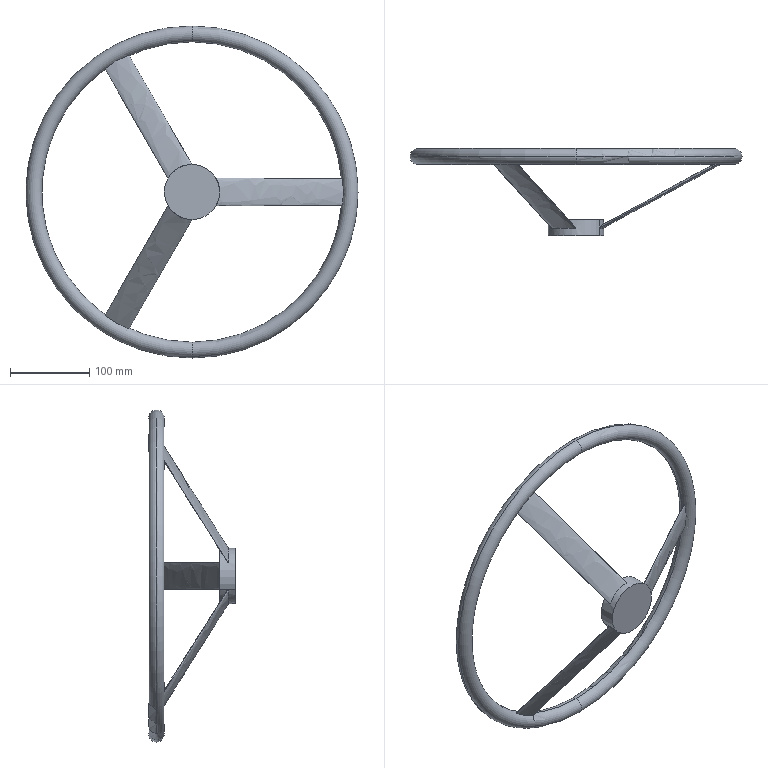Part | SolidWorks | 1 solid | 17 faces | box 420 x 110 x 420 mm | volume 545281 mm3 | spline 6 | plane 5 | torus 4 | cylinder 2 | commonest cylinder face diameters 70 x2
STEP:
#1=CARTESIAN_POINT('',(-101.45,99.061,160.701));
#2=VERTEX_POINT('',#1);
#3=CARTESIAN_POINT('',(-88.446,99.061,168.208));
#4=VERTEX_POINT('',#3);
#5=CARTESIAN_POINT('',(-101.45,99.061,160.701));
#6=CARTESIAN_POINT('',(-100.399,98.952,161.376));
#7=CARTESIAN_POINT('',(-99.34,98.865,162.042));
#8=CARTESIAN_POINT('',(-97.203,98.749,163.349));
#9=CARTESIAN_POINT('',(-96.124,98.719,163.991));
#10=CARTESIAN_POINT('',(-92.865,98.719,165.873));
#11=CARTESIAN_POINT('',(-90.666,98.842,167.065));
#12=CARTESIAN_POINT('',(-88.446,99.061,168.208));
#13=B_SPLINE_CURVE_WITH_KNOTS('',3,(#5,#6,#7,#8,#9,#10,#11,#12),.UNSPECIFIED.,.F.,.F.,(4,2,2,4),(0.002179,0.00594,0.009701,0.01722),.UNSPECIFIED.);
#14=EDGE_CURVE('',#2,#4,#13,.T.);
#15=ORIENTED_EDGE('',*,*,#14,.F.);
#16=CARTESIAN_POINT('',(-110.077,96.46,155.659));
#17=VERTEX_POINT('',#16);
#18=CARTESIAN_POINT('',(-110.077,96.46,155.659));
#19=CARTESIAN_POINT('',(-110.067,96.511,155.642));
#20=CARTESIAN_POINT('',(-110.046,96.564,155.633));
#21=CARTESIAN_POINT('',(-109.992,96.661,155.628));
#22=CARTESIAN_POINT('',(-109.959,96.706,155.632));
#23=CARTESIAN_POINT('',(-109.851,96.831,155.656));
#24=CARTESIAN_POINT('',(-109.769,96.901,155.686));
#25=CARTESIAN_POINT('',(-109.519,97.09,155.788));
#26=CARTESIAN_POINT('',(-109.341,97.191,155.877));
#27=CARTESIAN_POINT('',(-108.808,97.463,156.156));
#28=CARTESIAN_POINT('',(-108.445,97.604,156.366));
#29=CARTESIAN_POINT('',(-107.718,97.857,156.796));
#30=CARTESIAN_POINT('',(-107.354,97.967,157.018));
#31=CARTESIAN_POINT('',(-106.623,98.167,157.467));
#32=CARTESIAN_POINT('',(-106.256,98.257,157.695));
#33=CARTESIAN_POINT('',(-105.155,98.506,158.383));
#34=CARTESIAN_POINT('',(-104.418,98.644,158.847));
#35=CARTESIAN_POINT('',(-102.939,98.88,159.775));
#36=CARTESIAN_POINT('',(-102.196,98.979,160.239));
#37=CARTESIAN_POINT('',(-101.45,99.061,160.701));
#38=B_SPLINE_CURVE_WITH_KNOTS('',3,(#18,#19,#20,#21,#22,#23,#24,#25,#26,#27,#28,#29,#30,#31,#32,#33,#34,#35,#36,#37),.UNSPECIFIED.,.F.,.F.,(4,2,2,2,2,2,2,2,2,4),(0.04636,0.04653,0.04669,0.04702,0.04768,0.049,0.05032,0.05164,0.05428,0.05692),.UNSPECIFIED.);
#39=EDGE_CURVE('',#17,#2,#38,.T.);
#40=ORIENTED_EDGE('',*,*,#39,.F.);
#41=CARTESIAN_POINT('',(-79.766,96.46,173.159));
#42=VERTEX_POINT('',#41);
#43=CARTESIAN_POINT('',(-79.766,96.46,173.159));
#44=CARTESIAN_POINT('',(-79.783,96.371,173.188));
#45=CARTESIAN_POINT('',(-79.837,96.286,173.2));
#46=CARTESIAN_POINT('',(-79.968,96.149,173.201));
#47=CARTESIAN_POINT('',(-80.045,96.092,173.192));
#48=CARTESIAN_POINT('',(-80.282,95.943,173.153));
#49=CARTESIAN_POINT('',(-80.453,95.869,173.111));
#50=CARTESIAN_POINT('',(-80.963,95.674,172.973));
#51=CARTESIAN_POINT('',(-81.309,95.584,172.86));
#52=CARTESIAN_POINT('',(-82.001,95.425,172.621));
#53=CARTESIAN_POINT('',(-82.349,95.36,172.493));
#54=CARTESIAN_POINT('',(-83.042,95.245,172.228));
#55=CARTESIAN_POINT('',(-83.388,95.196,172.091));
#56=CARTESIAN_POINT('',(-84.424,95.062,171.669));
#57=CARTESIAN_POINT('',(-85.111,94.992,171.374));
#58=CARTESIAN_POINT('',(-86.479,94.875,170.765));
#59=CARTESIAN_POINT('',(-87.159,94.827,170.451));
#60=CARTESIAN_POINT('',(-89.191,94.707,169.486));
#61=CARTESIAN_POINT('',(-90.532,94.655,168.81));
#62=CARTESIAN_POINT('',(-93.188,94.587,167.409));
#63=CARTESIAN_POINT('',(-94.502,94.571,166.682));
#64=CARTESIAN_POINT('',(-97.103,94.571,165.18));
#65=CARTESIAN_POINT('',(-98.39,94.587,164.405));
#66=CARTESIAN_POINT('',(-100.931,94.655,162.806));
#67=CARTESIAN_POINT('',(-102.187,94.707,161.982));
#68=CARTESIAN_POINT('',(-104.039,94.828,160.706));
#69=CARTESIAN_POINT('',(-104.651,94.875,160.273));
#70=CARTESIAN_POINT('',(-105.862,94.993,159.393));
#71=CARTESIAN_POINT('',(-106.46,95.062,158.946));
#72=CARTESIAN_POINT('',(-107.344,95.196,158.26));
#73=CARTESIAN_POINT('',(-107.636,95.246,158.028));
#74=CARTESIAN_POINT('',(-108.212,95.361,157.56));
#75=CARTESIAN_POINT('',(-108.496,95.426,157.323));
#76=CARTESIAN_POINT('',(-108.912,95.545,156.962));
#77=CARTESIAN_POINT('',(-109.048,95.588,156.841));
#78=CARTESIAN_POINT('',(-109.316,95.687,156.597));
#79=CARTESIAN_POINT('',(-109.447,95.741,156.474));
#80=CARTESIAN_POINT('',(-109.697,95.871,156.225));
#81=CARTESIAN_POINT('',(-109.817,95.945,156.099));
#82=CARTESIAN_POINT('',(-109.969,96.095,155.914));
#83=CARTESIAN_POINT('',(-110.015,96.152,155.852));
#84=CARTESIAN_POINT('',(-110.078,96.288,155.74));
#85=CARTESIAN_POINT('',(-110.094,96.372,155.688));
#86=CARTESIAN_POINT('',(-110.077,96.46,155.659));
#87=B_SPLINE_CURVE_WITH_KNOTS('',3,(#43,#44,#45,#46,#47,#48,#49,#50,#51,#52,#53,#54,#55,#56,#57,#58,#59,#60,#61,#62,#63,#64,#65,#66,#67,#68,#69,#70,#71,#72,#73,#74,#75,#76,#77,#78,#79,#80,#81,#82,#83,#84,#85,#86),.UNSPECIFIED.,.F.,.F.,(4,2,2,2,2,2,2,2,2,2,2,2,2,2,2,2,2,2,2,2,2,4),(0.01057,0.01085,0.01113,0.01169,0.01281,0.01393,0.01505,0.01728,0.01952,0.02399,0.02847,0.03294,0.03742,0.03965,0.04189,0.04301,0.04413,0.04469,0.04525,0.04581,0.04609,0.04636),.UNSPECIFIED.);
#88=EDGE_CURVE('',#42,#17,#87,.T.);
#89=ORIENTED_EDGE('',*,*,#88,.F.);
#90=CARTESIAN_POINT('',(-88.446,99.061,168.208));
#91=CARTESIAN_POINT('',(-87.673,98.979,168.624));
#92=CARTESIAN_POINT('',(-86.9,98.88,169.035));
#93=CARTESIAN_POINT('',(-85.357,98.644,169.852));
#94=CARTESIAN_POINT('',(-84.587,98.506,170.258));
#95=CARTESIAN_POINT('',(-83.441,98.258,170.868));
#96=CARTESIAN_POINT('',(-83.061,98.167,171.071));
#97=CARTESIAN_POINT('',(-82.306,97.967,171.479));
#98=CARTESIAN_POINT('',(-81.931,97.857,171.684));
#99=CARTESIAN_POINT('',(-81.381,97.668,171.994));
#100=CARTESIAN_POINT('',(-81.199,97.601,172.098));
#101=CARTESIAN_POINT('',(-80.841,97.453,172.308));
#102=CARTESIAN_POINT('',(-80.664,97.373,172.415));
#103=CARTESIAN_POINT('',(-80.325,97.192,172.629));
#104=CARTESIAN_POINT('',(-80.162,97.093,172.737));
#105=CARTESIAN_POINT('',(-79.947,96.904,172.903));
#106=CARTESIAN_POINT('',(-79.879,96.833,172.96));
#107=CARTESIAN_POINT('',(-79.803,96.709,173.042));
#108=CARTESIAN_POINT('',(-79.783,96.663,173.069));
#109=CARTESIAN_POINT('',(-79.759,96.565,173.119));
#110=CARTESIAN_POINT('',(-79.756,96.512,173.141));
#111=CARTESIAN_POINT('',(-79.766,96.46,173.159));
#112=B_SPLINE_CURVE_WITH_KNOTS('',3,(#90,#91,#92,#93,#94,#95,#96,#97,#98,#99,#100,#101,#102,#103,#104,#105,#106,#107,#108,#109,#110,#111),.UNSPECIFIED.,.F.,.F.,(4,2,2,2,2,2,2,2,2,2,4),(0.,0.002643,0.005286,0.006608,0.00793,0.008591,0.009251,0.009912,0.01024,0.01041,0.01057),.UNSPECIFIED.);
#113=EDGE_CURVE('',#4,#42,#112,.T.);
#114=ORIENTED_EDGE('',*,*,#113,.F.);
#115=EDGE_LOOP('',(#15,#40,#89,#114));
#116=FACE_BOUND('',#115,.T.);
#117=CARTESIAN_POINT('',(-88.446,99.061,-168.208));
#118=VERTEX_POINT('',#117);
#119=CARTESIAN_POINT('',(-101.45,99.061,-160.701));
#120=VERTEX_POINT('',#119);
#121=CARTESIAN_POINT('',(-88.446,99.061,-168.208));
#122=CARTESIAN_POINT('',(-89.557,98.952,-167.636));
#123=CARTESIAN_POINT('',(-90.662,98.865,-167.052));
#124=CARTESIAN_POINT('',(-92.863,98.749,-165.855));
#125=CARTESIAN_POINT('',(-93.959,98.719,-165.241));
#126=CARTESIAN_POINT('',(-97.217,98.719,-163.36));
#127=CARTESIAN_POINT('',(-99.349,98.842,-162.051));
#128=CARTESIAN_POINT('',(-101.45,99.061,-160.701));
#129=B_SPLINE_CURVE_WITH_KNOTS('',3,(#121,#122,#123,#124,#125,#126,#127,#128),.UNSPECIFIED.,.F.,.F.,(4,2,2,4),(0.002179,0.00594,0.009701,0.01722),.UNSPECIFIED.);
#130=EDGE_CURVE('',#118,#120,#129,.T.);
#131=ORIENTED_EDGE('',*,*,#130,.F.);
#132=CARTESIAN_POINT('',(-79.766,96.46,-173.159));
#133=VERTEX_POINT('',#132);
#134=CARTESIAN_POINT('',(-79.766,96.46,-173.159));
#135=CARTESIAN_POINT('',(-79.756,96.511,-173.142));
#136=CARTESIAN_POINT('',(-79.759,96.564,-173.119));
#137=CARTESIAN_POINT('',(-79.782,96.661,-173.07));
#138=CARTESIAN_POINT('',(-79.802,96.706,-173.043));
#139=CARTESIAN_POINT('',(-79.877,96.831,-172.962));
#140=CARTESIAN_POINT('',(-79.943,96.901,-172.905));
#141=CARTESIAN_POINT('',(-80.157,97.09,-172.74));
#142=CARTESIAN_POINT('',(-80.323,97.191,-172.63));
#143=CARTESIAN_POINT('',(-80.831,97.463,-172.308));
#144=CARTESIAN_POINT('',(-81.195,97.604,-172.099));
#145=CARTESIAN_POINT('',(-81.93,97.857,-171.685));
#146=CARTESIAN_POINT('',(-82.304,97.967,-171.48));
#147=CARTESIAN_POINT('',(-83.059,98.167,-171.072));
#148=CARTESIAN_POINT('',(-83.44,98.257,-170.868));
#149=CARTESIAN_POINT('',(-84.586,98.506,-170.259));
#150=CARTESIAN_POINT('',(-85.357,98.644,-169.852));
#151=CARTESIAN_POINT('',(-86.9,98.88,-169.035));
#152=CARTESIAN_POINT('',(-87.673,98.979,-168.624));
#153=CARTESIAN_POINT('',(-88.446,99.061,-168.208));
#154=B_SPLINE_CURVE_WITH_KNOTS('',3,(#134,#135,#136,#137,#138,#139,#140,#141,#142,#143,#144,#145,#146,#147,#148,#149,#150,#151,#152,#153),.UNSPECIFIED.,.F.,.F.,(4,2,2,2,2,2,2,2,2,4),(0.04636,0.04653,0.04669,0.04702,0.04768,0.049,0.05032,0.05164,0.05428,0.05692),.UNSPECIFIED.);
#155=EDGE_CURVE('',#133,#118,#154,.T.);
#156=ORIENTED_EDGE('',*,*,#155,.F.);
#157=CARTESIAN_POINT('',(-110.077,96.46,-155.659));
#158=VERTEX_POINT('',#157);
#159=CARTESIAN_POINT('',(-110.077,96.46,-155.659));
#160=CARTESIAN_POINT('',(-110.094,96.371,-155.688));
#161=CARTESIAN_POINT('',(-110.077,96.286,-155.741));
#162=CARTESIAN_POINT('',(-110.013,96.149,-155.855));
#163=CARTESIAN_POINT('',(-109.966,96.092,-155.917));
#164=CARTESIAN_POINT('',(-109.814,95.943,-156.103));
#165=CARTESIAN_POINT('',(-109.692,95.869,-156.23));
#166=CARTESIAN_POINT('',(-109.317,95.674,-156.603));
#167=CARTESIAN_POINT('',(-109.047,95.584,-156.845));
#168=CARTESIAN_POINT('',(-108.494,95.425,-157.325));
#169=CARTESIAN_POINT('',(-108.209,95.36,-157.563));
#170=CARTESIAN_POINT('',(-107.633,95.245,-158.03));
#171=CARTESIAN_POINT('',(-107.341,95.196,-158.262));
#172=CARTESIAN_POINT('',(-106.458,95.062,-158.948));
#173=CARTESIAN_POINT('',(-105.859,94.992,-159.396));
#174=CARTESIAN_POINT('',(-104.648,94.875,-160.276));
#175=CARTESIAN_POINT('',(-104.035,94.827,-160.708));
#176=CARTESIAN_POINT('',(-102.184,94.707,-161.984));
#177=CARTESIAN_POINT('',(-100.928,94.655,-162.808));
#178=CARTESIAN_POINT('',(-98.386,94.587,-164.407));
#179=CARTESIAN_POINT('',(-97.1,94.571,-165.182));
#180=CARTESIAN_POINT('',(-94.499,94.571,-166.684));
#181=CARTESIAN_POINT('',(-93.184,94.587,-167.411));
#182=CARTESIAN_POINT('',(-90.528,94.655,-168.812));
#183=CARTESIAN_POINT('',(-89.187,94.707,-169.487));
#184=CARTESIAN_POINT('',(-87.156,94.828,-170.453));
#185=CARTESIAN_POINT('',(-86.475,94.875,-170.767));
#186=CARTESIAN_POINT('',(-85.108,94.993,-171.376));
#187=CARTESIAN_POINT('',(-84.421,95.062,-171.67));
#188=CARTESIAN_POINT('',(-83.385,95.196,-172.092));
#189=CARTESIAN_POINT('',(-83.039,95.246,-172.229));
#190=CARTESIAN_POINT('',(-82.345,95.361,-172.494));
#191=CARTESIAN_POINT('',(-81.998,95.426,-172.622));
#192=CARTESIAN_POINT('',(-81.478,95.545,-172.802));
#193=CARTESIAN_POINT('',(-81.304,95.588,-172.859));
#194=CARTESIAN_POINT('',(-80.959,95.687,-172.969));
#195=CARTESIAN_POINT('',(-80.787,95.741,-173.021));
#196=CARTESIAN_POINT('',(-80.446,95.871,-173.113));
#197=CARTESIAN_POINT('',(-80.277,95.945,-173.154));
#198=CARTESIAN_POINT('',(-80.041,96.095,-173.193));
#199=CARTESIAN_POINT('',(-79.965,96.152,-173.202));
#200=CARTESIAN_POINT('',(-79.836,96.288,-173.2));
#201=CARTESIAN_POINT('',(-79.783,96.372,-173.188));
#202=CARTESIAN_POINT('',(-79.766,96.46,-173.159));
#203=B_SPLINE_CURVE_WITH_KNOTS('',3,(#159,#160,#161,#162,#163,#164,#165,#166,#167,#168,#169,#170,#171,#172,#173,#174,#175,#176,#177,#178,#179,#180,#181,#182,#183,#184,#185,#186,#187,#188,#189,#190,#191,#192,#193,#194,#195,#196,#197,#198,#199,#200,#201,#202),.UNSPECIFIED.,.F.,.F.,(4,2,2,2,2,2,2,2,2,2,2,2,2,2,2,2,2,2,2,2,2,4),(0.01057,0.01085,0.01113,0.01169,0.01281,0.01393,0.01505,0.01728,0.01952,0.02399,0.02847,0.03294,0.03742,0.03965,0.04189,0.04301,0.04413,0.04469,0.04525,0.04581,0.04609,0.04636),.UNSPECIFIED.);
#204=EDGE_CURVE('',#158,#133,#203,.T.);
#205=ORIENTED_EDGE('',*,*,#204,.F.);
#206=CARTESIAN_POINT('',(-101.45,99.061,-160.701));
#207=CARTESIAN_POINT('',(-102.196,98.979,-160.239));
#208=CARTESIAN_POINT('',(-102.938,98.88,-159.775));
#209=CARTESIAN_POINT('',(-104.418,98.644,-158.847));
#210=CARTESIAN_POINT('',(-105.155,98.506,-158.383));
#211=CARTESIAN_POINT('',(-106.256,98.258,-157.696));
#212=CARTESIAN_POINT('',(-106.622,98.167,-157.468));
#213=CARTESIAN_POINT('',(-107.353,97.967,-157.018));
#214=CARTESIAN_POINT('',(-107.717,97.857,-156.797));
#215=CARTESIAN_POINT('',(-108.261,97.668,-156.475));
#216=CARTESIAN_POINT('',(-108.442,97.601,-156.369));
#217=CARTESIAN_POINT('',(-108.803,97.453,-156.164));
#218=CARTESIAN_POINT('',(-108.983,97.373,-156.064));
#219=CARTESIAN_POINT('',(-109.338,97.192,-155.878));
#220=CARTESIAN_POINT('',(-109.513,97.093,-155.791));
#221=CARTESIAN_POINT('',(-109.765,96.904,-155.687));
#222=CARTESIAN_POINT('',(-109.848,96.833,-155.657));
#223=CARTESIAN_POINT('',(-109.957,96.709,-155.633));
#224=CARTESIAN_POINT('',(-109.991,96.663,-155.628));
#225=CARTESIAN_POINT('',(-110.046,96.565,-155.632));
#226=CARTESIAN_POINT('',(-110.067,96.512,-155.641));
#227=CARTESIAN_POINT('',(-110.077,96.46,-155.659));
#228=B_SPLINE_CURVE_WITH_KNOTS('',3,(#206,#207,#208,#209,#210,#211,#212,#213,#214,#215,#216,#217,#218,#219,#220,#221,#222,#223,#224,#225,#226,#227),.UNSPECIFIED.,.F.,.F.,(4,2,2,2,2,2,2,2,2,2,4),(0.,0.002643,0.005286,0.006608,0.00793,0.008591,0.009251,0.009912,0.01024,0.01041,0.01057),.UNSPECIFIED.);
#229=EDGE_CURVE('',#120,#158,#228,.T.);
#230=ORIENTED_EDGE('',*,*,#229,.F.);
#231=EDGE_LOOP('',(#131,#156,#205,#230));
#232=FACE_BOUND('',#231,.T.);
#233=CARTESIAN_POINT('',(0.,100.,210.));
#234=VERTEX_POINT('',#233);
#235=CARTESIAN_POINT('',(0.,100.,190.));
#236=VERTEX_POINT('',#235);
#237=CARTESIAN_POINT('',(0.,100.,200.));
#238=DIRECTION('',(1.,0.,0.));
#239=DIRECTION('',(0.,0.,-1.));
#240=AXIS2_PLACEMENT_3D('',#237,#238,#239);
#241=CIRCLE('',#240,10.);
#242=EDGE_CURVE('',#234,#236,#241,.T.);
#243=ORIENTED_EDGE('',*,*,#242,.F.);
#244=CARTESIAN_POINT('',(0.,100.,-210.));
#245=VERTEX_POINT('',#244);
#246=CARTESIAN_POINT('',(0.,100.,0.));
#247=DIRECTION('',(0.,-1.,0.));
#248=DIRECTION('',(0.,0.,-1.));
#249=AXIS2_PLACEMENT_3D('',#246,#247,#248);
#250=CIRCLE('',#249,210.);
#251=EDGE_CURVE('',#234,#245,#250,.T.);
#252=ORIENTED_EDGE('',*,*,#251,.T.);
#253=CARTESIAN_POINT('',(0.,100.,-190.));
#254=VERTEX_POINT('',#253);
#255=CARTESIAN_POINT('',(0.,100.,-200.));
#256=DIRECTION('',(-1.,0.,0.));
#257=DIRECTION('',(0.,0.,1.));
#258=AXIS2_PLACEMENT_3D('',#255,#256,#257);
#259=CIRCLE('',#258,10.);
#260=EDGE_CURVE('',#245,#254,#259,.T.);
#261=ORIENTED_EDGE('',*,*,#260,.T.);
#262=CARTESIAN_POINT('',(0.,100.,0.));
#263=DIRECTION('',(0.,-1.,0.));
#264=DIRECTION('',(0.,0.,-1.));
#265=AXIS2_PLACEMENT_3D('',#262,#263,#264);
#266=CIRCLE('',#265,190.);
#267=EDGE_CURVE('',#236,#254,#266,.T.);
#268=ORIENTED_EDGE('',*,*,#267,.F.);
#269=EDGE_LOOP('',(#243,#252,#261,#268));
#270=FACE_OUTER_BOUND('',#269,.T.);
#271=CARTESIAN_POINT('',(0.,100.,0.));
#272=DIRECTION('',(0.,-1.,0.));
#273=DIRECTION('',(0.,0.,-1.));
#274=AXIS2_PLACEMENT_3D('',#271,#272,#273);
#275=TOROIDAL_SURFACE('',#274,200.,10.);
#276=ADVANCED_FACE('',(#116,#232,#270),#275,.T.);
#277=CARTESIAN_POINT('',(189.896,99.061,7.508));
#278=VERTEX_POINT('',#277);
#279=CARTESIAN_POINT('',(189.896,99.061,-7.508));
#280=VERTEX_POINT('',#279);
#281=CARTESIAN_POINT('',(189.896,99.061,7.508));
#282=CARTESIAN_POINT('',(189.955,98.952,6.26));
#283=CARTESIAN_POINT('',(190.002,98.865,5.01));
#284=CARTESIAN_POINT('',(190.066,98.749,2.506));
#285=CARTESIAN_POINT('',(190.082,98.719,1.25));
#286=CARTESIAN_POINT('',(190.082,98.719,-2.513));
#287=CARTESIAN_POINT('',(190.015,98.842,-5.013));
#288=CARTESIAN_POINT('',(189.896,99.061,-7.508));
#289=B_SPLINE_CURVE_WITH_KNOTS('',3,(#281,#282,#283,#284,#285,#286,#287,#288),.UNSPECIFIED.,.F.,.F.,(4,2,2,4),(0.002179,0.00594,0.009701,0.01722),.UNSPECIFIED.);
#290=EDGE_CURVE('',#278,#280,#289,.T.);
#291=ORIENTED_EDGE('',*,*,#290,.F.);
#292=CARTESIAN_POINT('',(189.843,96.46,17.5));
#293=VERTEX_POINT('',#292);
#294=CARTESIAN_POINT('',(189.843,96.46,17.5));
#295=CARTESIAN_POINT('',(189.823,96.511,17.5));
#296=CARTESIAN_POINT('',(189.805,96.564,17.487));
#297=CARTESIAN_POINT('',(189.774,96.661,17.442));
#298=CARTESIAN_POINT('',(189.761,96.706,17.411));
#299=CARTESIAN_POINT('',(189.727,96.831,17.306));
#300=CARTESIAN_POINT('',(189.712,96.901,17.22));
#301=CARTESIAN_POINT('',(189.676,97.09,16.952));
#302=CARTESIAN_POINT('',(189.664,97.191,16.754));
#303=CARTESIAN_POINT('',(189.639,97.463,16.152));
#304=CARTESIAN_POINT('',(189.639,97.604,15.733));
#305=CARTESIAN_POINT('',(189.648,97.857,14.889));
#306=CARTESIAN_POINT('',(189.658,97.967,14.462));
#307=CARTESIAN_POINT('',(189.682,98.167,13.604));
#308=CARTESIAN_POINT('',(189.696,98.257,13.173));
#309=CARTESIAN_POINT('',(189.741,98.506,11.876));
#310=CARTESIAN_POINT('',(189.775,98.644,11.005));
#311=CARTESIAN_POINT('',(189.838,98.88,9.26));
#312=CARTESIAN_POINT('',(189.869,98.979,8.385));
#313=CARTESIAN_POINT('',(189.896,99.061,7.508));
#314=B_SPLINE_CURVE_WITH_KNOTS('',3,(#294,#295,#296,#297,#298,#299,#300,#301,#302,#303,#304,#305,#306,#307,#308,#309,#310,#311,#312,#313),.UNSPECIFIED.,.F.,.F.,(4,2,2,2,2,2,2,2,2,4),(0.04636,0.04653,0.04669,0.04702,0.04768,0.049,0.05032,0.05164,0.05428,0.05692),.UNSPECIFIED.);
#315=EDGE_CURVE('',#293,#278,#314,.T.);
#316=ORIENTED_EDGE('',*,*,#315,.F.);
#317=CARTESIAN_POINT('',(189.843,96.46,-17.5));
#318=VERTEX_POINT('',#317);
#319=CARTESIAN_POINT('',(189.843,96.46,-17.5));
#320=CARTESIAN_POINT('',(189.876,96.371,-17.5));
#321=CARTESIAN_POINT('',(189.914,96.286,-17.459));
#322=CARTESIAN_POINT('',(189.981,96.149,-17.347));
#323=CARTESIAN_POINT('',(190.011,96.092,-17.275));
#324=CARTESIAN_POINT('',(190.096,95.943,-17.051));
#325=CARTESIAN_POINT('',(190.145,95.869,-16.882));
#326=CARTESIAN_POINT('',(190.28,95.674,-16.37));
#327=CARTESIAN_POINT('',(190.355,95.584,-16.015));
#328=CARTESIAN_POINT('',(190.495,95.425,-15.295));
#329=CARTESIAN_POINT('',(190.558,95.36,-14.93));
#330=CARTESIAN_POINT('',(190.675,95.245,-14.198));
#331=CARTESIAN_POINT('',(190.729,95.196,-13.83));
#332=CARTESIAN_POINT('',(190.882,95.062,-12.721));
#333=CARTESIAN_POINT('',(190.97,94.992,-11.979));
#334=CARTESIAN_POINT('',(191.127,94.875,-10.49));
#335=CARTESIAN_POINT('',(191.195,94.827,-9.743));
#336=CARTESIAN_POINT('',(191.374,94.707,-7.501));
#337=CARTESIAN_POINT('',(191.46,94.655,-6.002));
#338=CARTESIAN_POINT('',(191.574,94.587,-3.002));
#339=CARTESIAN_POINT('',(191.602,94.571,-1.5));
#340=CARTESIAN_POINT('',(191.602,94.571,1.504));
#341=CARTESIAN_POINT('',(191.574,94.587,3.006));
#342=CARTESIAN_POINT('',(191.46,94.655,6.006));
#343=CARTESIAN_POINT('',(191.374,94.707,7.505));
#344=CARTESIAN_POINT('',(191.195,94.828,9.747));
#345=CARTESIAN_POINT('',(191.126,94.875,10.494));
#346=CARTESIAN_POINT('',(190.97,94.993,11.982));
#347=CARTESIAN_POINT('',(190.881,95.062,12.724));
#348=CARTESIAN_POINT('',(190.729,95.196,13.832));
#349=CARTESIAN_POINT('',(190.674,95.246,14.201));
#350=CARTESIAN_POINT('',(190.557,95.361,14.934));
#351=CARTESIAN_POINT('',(190.494,95.426,15.299));
#352=CARTESIAN_POINT('',(190.389,95.545,15.839));
#353=CARTESIAN_POINT('',(190.353,95.588,16.018));
#354=CARTESIAN_POINT('',(190.275,95.687,16.372));
#355=CARTESIAN_POINT('',(190.234,95.741,16.547));
#356=CARTESIAN_POINT('',(190.143,95.871,16.888));
#357=CARTESIAN_POINT('',(190.095,95.945,17.055));
#358=CARTESIAN_POINT('',(190.01,96.095,17.279));
#359=CARTESIAN_POINT('',(189.979,96.152,17.35));
#360=CARTESIAN_POINT('',(189.913,96.288,17.46));
#361=CARTESIAN_POINT('',(189.876,96.372,17.5));
#362=CARTESIAN_POINT('',(189.843,96.46,17.5));
#363=B_SPLINE_CURVE_WITH_KNOTS('',3,(#319,#320,#321,#322,#323,#324,#325,#326,#327,#328,#329,#330,#331,#332,#333,#334,#335,#336,#337,#338,#339,#340,#341,#342,#343,#344,#345,#346,#347,#348,#349,#350,#351,#352,#353,#354,#355,#356,#357,#358,#359,#360,#361,#362),.UNSPECIFIED.,.F.,.F.,(4,2,2,2,2,2,2,2,2,2,2,2,2,2,2,2,2,2,2,2,2,4),(0.01057,0.01085,0.01113,0.01169,0.01281,0.01393,0.01505,0.01728,0.01952,0.02399,0.02847,0.03294,0.03742,0.03965,0.04189,0.04301,0.04413,0.04469,0.04525,0.04581,0.04609,0.04636),.UNSPECIFIED.);
#364=EDGE_CURVE('',#318,#293,#363,.T.);
#365=ORIENTED_EDGE('',*,*,#364,.F.);
#366=CARTESIAN_POINT('',(189.896,99.061,-7.508));
#367=CARTESIAN_POINT('',(189.869,98.979,-8.385));
#368=CARTESIAN_POINT('',(189.839,98.88,-9.26));
#369=CARTESIAN_POINT('',(189.775,98.644,-11.005));
#370=CARTESIAN_POINT('',(189.741,98.506,-11.875));
#371=CARTESIAN_POINT('',(189.696,98.258,-13.172));
#372=CARTESIAN_POINT('',(189.682,98.167,-13.603));
#373=CARTESIAN_POINT('',(189.658,97.967,-14.461));
#374=CARTESIAN_POINT('',(189.648,97.857,-14.887));
#375=CARTESIAN_POINT('',(189.642,97.668,-15.519));
#376=CARTESIAN_POINT('',(189.641,97.601,-15.729));
#377=CARTESIAN_POINT('',(189.644,97.453,-16.144));
#378=CARTESIAN_POINT('',(189.647,97.373,-16.35));
#379=CARTESIAN_POINT('',(189.664,97.192,-16.751));
#380=CARTESIAN_POINT('',(189.675,97.093,-16.946));
#381=CARTESIAN_POINT('',(189.711,96.904,-17.215));
#382=CARTESIAN_POINT('',(189.727,96.833,-17.303));
#383=CARTESIAN_POINT('',(189.76,96.709,-17.409));
#384=CARTESIAN_POINT('',(189.773,96.663,-17.441));
#385=CARTESIAN_POINT('',(189.804,96.565,-17.486));
#386=CARTESIAN_POINT('',(189.823,96.512,-17.5));
#387=CARTESIAN_POINT('',(189.843,96.46,-17.5));
#388=B_SPLINE_CURVE_WITH_KNOTS('',3,(#366,#367,#368,#369,#370,#371,#372,#373,#374,#375,#376,#377,#378,#379,#380,#381,#382,#383,#384,#385,#386,#387),.UNSPECIFIED.,.F.,.F.,(4,2,2,2,2,2,2,2,2,2,4),(0.,0.002643,0.005286,0.006608,0.00793,0.008591,0.009251,0.009912,0.01024,0.01041,0.01057),.UNSPECIFIED.);
#389=EDGE_CURVE('',#280,#318,#388,.T.);
#390=ORIENTED_EDGE('',*,*,#389,.F.);
#391=EDGE_LOOP('',(#291,#316,#365,#390));
#392=FACE_BOUND('',#391,.T.);
#393=ORIENTED_EDGE('',*,*,#260,.F.);
#394=CARTESIAN_POINT('',(0.,100.,0.));
#395=DIRECTION('',(0.,-1.,0.));
#396=DIRECTION('',(0.,0.,-1.));
#397=AXIS2_PLACEMENT_3D('',#394,#395,#396);
#398=CIRCLE('',#397,210.);
#399=EDGE_CURVE('',#245,#234,#398,.T.);
#400=ORIENTED_EDGE('',*,*,#399,.T.);
#401=ORIENTED_EDGE('',*,*,#242,.T.);
#402=CARTESIAN_POINT('',(0.,100.,0.));
#403=DIRECTION('',(0.,-1.,0.));
#404=DIRECTION('',(0.,0.,-1.));
#405=AXIS2_PLACEMENT_3D('',#402,#403,#404);
#406=CIRCLE('',#405,190.);
#407=EDGE_CURVE('',#254,#236,#406,.T.);
#408=ORIENTED_EDGE('',*,*,#407,.F.);
#409=EDGE_LOOP('',(#393,#400,#401,#408));
#410=FACE_OUTER_BOUND('',#409,.T.);
#411=CARTESIAN_POINT('',(0.,100.,0.));
#412=DIRECTION('',(0.,-1.,0.));
#413=DIRECTION('',(0.,0.,-1.));
#414=AXIS2_PLACEMENT_3D('',#411,#412,#413);
#415=TOROIDAL_SURFACE('',#414,200.,10.);
#416=ADVANCED_FACE('',(#392,#410),#415,.T.);
#417=CARTESIAN_POINT('',(0.,9.442,35.));
#418=VERTEX_POINT('',#417);
#419=CARTESIAN_POINT('',(-30.311,9.442,17.5));
#420=VERTEX_POINT('',#419);
#421=CARTESIAN_POINT('',(0.,9.442,35.));
#422=CARTESIAN_POINT('',(0.,9.547,35.));
#423=CARTESIAN_POINT('',(-0.03924,9.646,35.));
#424=CARTESIAN_POINT('',(-0.1408,9.825,35.));
#425=CARTESIAN_POINT('',(-0.2051,9.907,34.999));
#426=CARTESIAN_POINT('',(-0.4098,10.137,34.998));
#427=CARTESIAN_POINT('',(-0.5645,10.27,34.996));
#428=CARTESIAN_POINT('',(-1.049,10.647,34.986));
#429=CARTESIAN_POINT('',(-1.397,10.864,34.974));
#430=CARTESIAN_POINT('',(-2.105,11.269,34.938));
#431=CARTESIAN_POINT('',(-2.469,11.456,34.915));
#432=CARTESIAN_POINT('',(-3.205,11.809,34.855));
#433=CARTESIAN_POINT('',(-3.577,11.974,34.819));
#434=CARTESIAN_POINT('',(-4.704,12.445,34.691));
#435=CARTESIAN_POINT('',(-5.465,12.724,34.579));
#436=CARTESIAN_POINT('',(-6.993,13.228,34.303));
#437=CARTESIAN_POINT('',(-7.763,13.454,34.137));
#438=CARTESIAN_POINT('',(-9.3,13.853,33.751));
#439=CARTESIAN_POINT('',(-10.067,14.026,33.531));
#440=CARTESIAN_POINT('',(-11.595,14.325,33.033));
#441=CARTESIAN_POINT('',(-12.356,14.449,32.757));
#442=CARTESIAN_POINT('',(-13.858,14.648,32.15));
#443=CARTESIAN_POINT('',(-14.603,14.723,31.818));
#444=CARTESIAN_POINT('',(-16.07,14.823,31.103));
#445=CARTESIAN_POINT('',(-16.791,14.848,30.72));
#446=CARTESIAN_POINT('',(-18.206,14.848,29.903));
#447=CARTESIAN_POINT('',(-18.901,14.823,29.469));
#448=CARTESIAN_POINT('',(-20.252,14.723,28.557));
#449=CARTESIAN_POINT('',(-20.91,14.649,28.079));
#450=CARTESIAN_POINT('',(-22.19,14.449,27.079));
#451=CARTESIAN_POINT('',(-22.808,14.325,26.56));
#452=CARTESIAN_POINT('',(-24.002,14.027,25.486));
#453=CARTESIAN_POINT('',(-24.579,13.853,24.93));
#454=CARTESIAN_POINT('',(-25.681,13.454,23.793));
#455=CARTESIAN_POINT('',(-26.208,13.23,23.211));
#456=CARTESIAN_POINT('',(-27.214,12.724,22.023));
#457=CARTESIAN_POINT('',(-27.692,12.444,21.418));
#458=CARTESIAN_POINT('',(-28.365,11.974,20.507));
#459=CARTESIAN_POINT('',(-28.583,11.809,20.203));
#460=CARTESIAN_POINT('',(-29.003,11.456,19.595));
#461=CARTESIAN_POINT('',(-29.205,11.269,19.292));
#462=CARTESIAN_POINT('',(-29.59,10.864,18.697));
#463=CARTESIAN_POINT('',(-29.774,10.646,18.401));
#464=CARTESIAN_POINT('',(-30.025,10.27,17.987));
#465=CARTESIAN_POINT('',(-30.104,10.137,17.854));
#466=CARTESIAN_POINT('',(-30.208,9.907,17.677));
#467=CARTESIAN_POINT('',(-30.24,9.825,17.622));
#468=CARTESIAN_POINT('',(-30.291,9.646,17.534));
#469=CARTESIAN_POINT('',(-30.311,9.545,17.5));
#470=CARTESIAN_POINT('',(-30.311,9.442,17.5));
#471=B_SPLINE_CURVE_WITH_KNOTS('',3,(#421,#422,#423,#424,#425,#426,#427,#428,#429,#430,#431,#432,#433,#434,#435,#436,#437,#438,#439,#440,#441,#442,#443,#444,#445,#446,#447,#448,#449,#450,#451,#452,#453,#454,#455,#456,#457,#458,#459,#460,#461,#462,#463,#464,#465,#466,#467,#468,#469,#470),.UNSPECIFIED.,.F.,.F.,(4,2,2,2,2,2,2,2,2,2,2,2,2,2,2,2,2,2,2,2,2,2,2,2,4),(0.,0.0003085,0.0006169,0.001234,0.002468,0.003702,0.004935,0.007403,0.009871,0.01234,0.01481,0.01727,0.01974,0.02221,0.02468,0.02714,0.02961,0.03208,0.03455,0.03578,0.03702,0.03825,0.03887,0.03917,0.03948),.UNSPECIFIED.);
#472=EDGE_CURVE('',#418,#420,#471,.T.);
#473=ORIENTED_EDGE('',*,*,#472,.T.);
#474=CARTESIAN_POINT('',(-3.158,-20.179,-29.531));
#475=DIRECTION('',(-0.4389,0.4789,0.7603));
#476=VECTOR('',#475,1000.);
#477=LINE('',#474,#476);
#478=EDGE_CURVE('',#420,#17,#477,.T.);
#479=ORIENTED_EDGE('',*,*,#478,.T.);
#480=ORIENTED_EDGE('',*,*,#39,.T.);
#481=CARTESIAN_POINT('',(-88.446,99.061,168.208));
#482=CARTESIAN_POINT('',(-92.553,99.349,165.656));
#483=CARTESIAN_POINT('',(-97.186,99.349,162.981));
#484=CARTESIAN_POINT('',(-101.45,99.061,160.701));
#485=(BOUNDED_CURVE()B_SPLINE_CURVE(3,(#481,#482,#483,#484),.UNSPECIFIED.,.F.,.F.)B_SPLINE_CURVE_WITH_KNOTS((4,4),(1.127,2.014),.UNSPECIFIED.)CURVE()GEOMETRIC_REPRESENTATION_ITEM()RATIONAL_B_SPLINE_CURVE((1.,0.9355,0.9355,1.))REPRESENTATION_ITEM(''));
#486=EDGE_CURVE('',#4,#2,#485,.T.);
#487=ORIENTED_EDGE('',*,*,#486,.F.);
#488=ORIENTED_EDGE('',*,*,#113,.T.);
#489=CARTESIAN_POINT('',(27.153,-20.179,-12.031));
#490=DIRECTION('',(-0.4389,0.4789,0.7603));
#491=VECTOR('',#490,1000.);
#492=LINE('',#489,#491);
#493=EDGE_CURVE('',#418,#42,#492,.T.);
#494=ORIENTED_EDGE('',*,*,#493,.F.);
#495=EDGE_LOOP('',(#473,#479,#480,#487,#488,#494));
#496=FACE_OUTER_BOUND('',#495,.T.);
#497=CARTESIAN_POINT('',(0.482,8.916,34.165));
#498=CARTESIAN_POINT('',(-80.333,97.078,174.141));
#499=CARTESIAN_POINT('',(1.679,13.306,32.092));
#500=CARTESIAN_POINT('',(-79.136,101.468,172.068));
#501=CARTESIAN_POINT('',(-28.632,13.306,14.592));
#502=CARTESIAN_POINT('',(-109.447,101.468,154.568));
#503=CARTESIAN_POINT('',(-29.829,8.916,16.665));
#504=CARTESIAN_POINT('',(-110.644,97.078,156.641));
#505=(BOUNDED_SURFACE()B_SPLINE_SURFACE(3,1,((#497,#498),(#499,#500),(#501,#502),(#503,#504)),.UNSPECIFIED.,.F.,.F.,.F.)B_SPLINE_SURFACE_WITH_KNOTS((4,4),(2,2),(0.,1.),(0.,1.),.UNSPECIFIED.)GEOMETRIC_REPRESENTATION_ITEM()RATIONAL_B_SPLINE_SURFACE(((1.,1.),(0.3333,0.3333),(0.3333,0.3333),(1.,1.)))REPRESENTATION_ITEM('')SURFACE());
#506=ADVANCED_FACE('',(#496),#505,.T.);
#507=CARTESIAN_POINT('',(-30.311,9.442,-17.5));
#508=VERTEX_POINT('',#507);
#509=CARTESIAN_POINT('',(0.,9.442,-35.));
#510=VERTEX_POINT('',#509);
#511=CARTESIAN_POINT('',(-30.311,9.442,-17.5));
#512=CARTESIAN_POINT('',(-30.311,9.547,-17.5));
#513=CARTESIAN_POINT('',(-30.291,9.646,-17.534));
#514=CARTESIAN_POINT('',(-30.24,9.825,-17.622));
#515=CARTESIAN_POINT('',(-30.208,9.907,-17.677));
#516=CARTESIAN_POINT('',(-30.104,10.137,-17.854));
#517=CARTESIAN_POINT('',(-30.025,10.27,-17.987));
#518=CARTESIAN_POINT('',(-29.774,10.647,-18.401));
#519=CARTESIAN_POINT('',(-29.59,10.864,-18.697));
#520=CARTESIAN_POINT('',(-29.205,11.269,-19.293));
#521=CARTESIAN_POINT('',(-29.002,11.456,-19.596));
#522=CARTESIAN_POINT('',(-28.583,11.809,-20.203));
#523=CARTESIAN_POINT('',(-28.365,11.974,-20.508));
#524=CARTESIAN_POINT('',(-27.691,12.445,-21.419));
#525=CARTESIAN_POINT('',(-27.214,12.724,-22.022));
#526=CARTESIAN_POINT('',(-26.211,13.228,-23.207));
#527=CARTESIAN_POINT('',(-25.683,13.454,-23.792));
#528=CARTESIAN_POINT('',(-24.579,13.853,-24.929));
#529=CARTESIAN_POINT('',(-24.005,14.026,-25.483));
#530=CARTESIAN_POINT('',(-22.81,14.325,-26.558));
#531=CARTESIAN_POINT('',(-22.19,14.449,-27.079));
#532=CARTESIAN_POINT('',(-20.913,14.648,-28.077));
#533=CARTESIAN_POINT('',(-20.254,14.723,-28.556));
#534=CARTESIAN_POINT('',(-18.901,14.823,-29.469));
#535=CARTESIAN_POINT('',(-18.209,14.848,-29.901));
#536=CARTESIAN_POINT('',(-16.794,14.848,-30.719));
#537=CARTESIAN_POINT('',(-16.071,14.823,-31.103));
#538=CARTESIAN_POINT('',(-14.606,14.723,-31.817));
#539=CARTESIAN_POINT('',(-13.862,14.649,-32.148));
#540=CARTESIAN_POINT('',(-12.356,14.449,-32.757));
#541=CARTESIAN_POINT('',(-11.597,14.325,-33.032));
#542=CARTESIAN_POINT('',(-10.07,14.027,-33.53));
#543=CARTESIAN_POINT('',(-9.3,13.853,-33.751));
#544=CARTESIAN_POINT('',(-7.764,13.454,-34.137));
#545=CARTESIAN_POINT('',(-6.997,13.23,-34.302));
#546=CARTESIAN_POINT('',(-5.465,12.724,-34.579));
#547=CARTESIAN_POINT('',(-4.703,12.444,-34.691));
#548=CARTESIAN_POINT('',(-3.577,11.974,-34.819));
#549=CARTESIAN_POINT('',(-3.205,11.809,-34.855));
#550=CARTESIAN_POINT('',(-2.469,11.456,-34.915));
#551=CARTESIAN_POINT('',(-2.105,11.269,-34.938));
#552=CARTESIAN_POINT('',(-1.397,10.864,-34.974));
#553=CARTESIAN_POINT('',(-1.048,10.646,-34.986));
#554=CARTESIAN_POINT('',(-0.5646,10.27,-34.996));
#555=CARTESIAN_POINT('',(-0.4099,10.137,-34.998));
#556=CARTESIAN_POINT('',(-0.2045,9.907,-34.999));
#557=CARTESIAN_POINT('',(-0.1407,9.825,-35.));
#558=CARTESIAN_POINT('',(-0.03904,9.646,-35.));
#559=CARTESIAN_POINT('',(0.,9.545,-35.));
#560=CARTESIAN_POINT('',(0.,9.442,-35.));
#561=B_SPLINE_CURVE_WITH_KNOTS('',3,(#511,#512,#513,#514,#515,#516,#517,#518,#519,#520,#521,#522,#523,#524,#525,#526,#527,#528,#529,#530,#531,#532,#533,#534,#535,#536,#537,#538,#539,#540,#541,#542,#543,#544,#545,#546,#547,#548,#549,#550,#551,#552,#553,#554,#555,#556,#557,#558,#559,#560),.UNSPECIFIED.,.F.,.F.,(4,2,2,2,2,2,2,2,2,2,2,2,2,2,2,2,2,2,2,2,2,2,2,2,4),(0.,0.0003085,0.0006169,0.001234,0.002468,0.003702,0.004935,0.007403,0.009871,0.01234,0.01481,0.01727,0.01974,0.02221,0.02468,0.02714,0.02961,0.03208,0.03455,0.03578,0.03702,0.03825,0.03887,0.03917,0.03948),.UNSPECIFIED.);
#562=EDGE_CURVE('',#508,#510,#561,.T.);
#563=ORIENTED_EDGE('',*,*,#562,.T.);
#564=CARTESIAN_POINT('',(27.153,-20.179,12.031));
#565=DIRECTION('',(-0.4389,0.4789,-0.7603));
#566=VECTOR('',#565,1000.);
#567=LINE('',#564,#566);
#568=EDGE_CURVE('',#510,#133,#567,.T.);
#569=ORIENTED_EDGE('',*,*,#568,.T.);
#570=ORIENTED_EDGE('',*,*,#155,.T.);
#571=CARTESIAN_POINT('',(-101.45,99.061,-160.701));
#572=CARTESIAN_POINT('',(-97.186,99.349,-162.981));
#573=CARTESIAN_POINT('',(-92.553,99.349,-165.656));
#574=CARTESIAN_POINT('',(-88.446,99.061,-168.208));
#575=(BOUNDED_CURVE()B_SPLINE_CURVE(3,(#571,#572,#573,#574),.UNSPECIFIED.,.F.,.F.)B_SPLINE_CURVE_WITH_KNOTS((4,4),(1.127,2.014),.UNSPECIFIED.)CURVE()GEOMETRIC_REPRESENTATION_ITEM()RATIONAL_B_SPLINE_CURVE((1.,0.9355,0.9355,1.))REPRESENTATION_ITEM(''));
#576=EDGE_CURVE('',#120,#118,#575,.T.);
#577=ORIENTED_EDGE('',*,*,#576,.F.);
#578=ORIENTED_EDGE('',*,*,#229,.T.);
#579=CARTESIAN_POINT('',(-3.158,-20.179,29.531));
#580=DIRECTION('',(-0.4389,0.4789,-0.7603));
#581=VECTOR('',#580,1000.);
#582=LINE('',#579,#581);
#583=EDGE_CURVE('',#508,#158,#582,.T.);
#584=ORIENTED_EDGE('',*,*,#583,.F.);
#585=EDGE_LOOP('',(#563,#569,#570,#577,#578,#584));
#586=FACE_OUTER_BOUND('',#585,.T.);
#587=CARTESIAN_POINT('',(-29.829,8.916,-16.665));
#588=CARTESIAN_POINT('',(-110.644,97.078,-156.641));
#589=CARTESIAN_POINT('',(-28.632,13.306,-14.592));
#590=CARTESIAN_POINT('',(-109.447,101.468,-154.568));
#591=CARTESIAN_POINT('',(1.679,13.306,-32.092));
#592=CARTESIAN_POINT('',(-79.136,101.468,-172.068));
#593=CARTESIAN_POINT('',(0.482,8.916,-34.165));
#594=CARTESIAN_POINT('',(-80.333,97.078,-174.141));
#595=(BOUNDED_SURFACE()B_SPLINE_SURFACE(3,1,((#587,#588),(#589,#590),(#591,#592),(#593,#594)),.UNSPECIFIED.,.F.,.F.,.F.)B_SPLINE_SURFACE_WITH_KNOTS((4,4),(2,2),(0.,1.),(0.,1.),.UNSPECIFIED.)GEOMETRIC_REPRESENTATION_ITEM()RATIONAL_B_SPLINE_SURFACE(((1.,1.),(0.3333,0.3333),(0.3333,0.3333),(1.,1.)))REPRESENTATION_ITEM('')SURFACE());
#596=ADVANCED_FACE('',(#586),#595,.T.);
#597=ORIENTED_EDGE('',*,*,#472,.F.);
#598=CARTESIAN_POINT('',(-30.311,9.442,17.5));
#599=CARTESIAN_POINT('',(-30.311,9.393,17.5));
#600=CARTESIAN_POINT('',(-30.306,9.344,17.508));
#601=CARTESIAN_POINT('',(-30.287,9.254,17.541));
#602=CARTESIAN_POINT('',(-30.273,9.212,17.566));
#603=CARTESIAN_POINT('',(-30.223,9.105,17.652));
#604=CARTESIAN_POINT('',(-30.18,9.052,17.725));
#605=CARTESIAN_POINT('',(-30.045,8.924,17.953));
#606=CARTESIAN_POINT('',(-29.949,8.876,18.114));
#607=CARTESIAN_POINT('',(-29.75,8.8,18.438));
#608=CARTESIAN_POINT('',(-29.648,8.775,18.602));
#609=CARTESIAN_POINT('',(-29.441,8.736,18.928));
#610=CARTESIAN_POINT('',(-29.336,8.723,19.09));
#611=CARTESIAN_POINT('',(-29.017,8.694,19.575));
#612=CARTESIAN_POINT('',(-28.798,8.689,19.895));
#613=CARTESIAN_POINT('',(-28.35,8.69,20.528));
#614=CARTESIAN_POINT('',(-28.121,8.698,20.841));
#615=CARTESIAN_POINT('',(-27.418,8.729,21.768));
#616=CARTESIAN_POINT('',(-26.93,8.763,22.369));
#617=CARTESIAN_POINT('',(-25.915,8.833,23.538));
#618=CARTESIAN_POINT('',(-25.387,8.871,24.106));
#619=CARTESIAN_POINT('',(-23.751,8.979,25.755));
#620=CARTESIAN_POINT('',(-22.586,9.043,26.782));
#621=CARTESIAN_POINT('',(-20.132,9.129,28.672));
#622=CARTESIAN_POINT('',(-18.841,9.152,29.537));
#623=CARTESIAN_POINT('',(-16.828,9.152,30.699));
#624=CARTESIAN_POINT('',(-16.143,9.147,31.065));
#625=CARTESIAN_POINT('',(-14.752,9.124,31.749));
#626=CARTESIAN_POINT('',(-14.046,9.107,32.067));
#627=CARTESIAN_POINT('',(-11.896,9.042,32.953));
#628=CARTESIAN_POINT('',(-10.425,8.978,33.447));
#629=CARTESIAN_POINT('',(-8.179,8.871,34.04));
#630=CARTESIAN_POINT('',(-7.424,8.833,34.212));
#631=CARTESIAN_POINT('',(-5.904,8.763,34.507));
#632=CARTESIAN_POINT('',(-5.138,8.729,34.629));
#633=CARTESIAN_POINT('',(-3.984,8.698,34.775));
#634=CARTESIAN_POINT('',(-3.598,8.69,34.817));
#635=CARTESIAN_POINT('',(-2.826,8.689,34.888));
#636=CARTESIAN_POINT('',(-2.439,8.694,34.917));
#637=CARTESIAN_POINT('',(-1.859,8.723,34.951));
#638=CARTESIAN_POINT('',(-1.666,8.736,34.961));
#639=CARTESIAN_POINT('',(-1.28,8.775,34.977));
#640=CARTESIAN_POINT('',(-1.088,8.801,34.984));
#641=CARTESIAN_POINT('',(-0.7076,8.878,34.993));
#642=CARTESIAN_POINT('',(-0.5185,8.926,34.997));
#643=CARTESIAN_POINT('',(-0.2566,9.054,34.999));
#644=CARTESIAN_POINT('',(-0.1726,9.107,35.));
#645=CARTESIAN_POINT('',(-0.0747,9.214,35.));
#646=CARTESIAN_POINT('',(-0.0468,9.255,35.));
#647=CARTESIAN_POINT('',(-0.009479,9.344,35.));
#648=CARTESIAN_POINT('',(0.,9.392,35.));
#649=CARTESIAN_POINT('',(0.,9.442,35.));
#650=B_SPLINE_CURVE_WITH_KNOTS('',3,(#598,#599,#600,#601,#602,#603,#604,#605,#606,#607,#608,#609,#610,#611,#612,#613,#614,#615,#616,#617,#618,#619,#620,#621,#622,#623,#624,#625,#626,#627,#628,#629,#630,#631,#632,#633,#634,#635,#636,#637,#638,#639,#640,#641,#642,#643,#644,#645,#646,#647,#648,#649),.UNSPECIFIED.,.F.,.F.,(4,2,2,2,2,2,2,2,2,2,2,2,2,2,2,2,2,2,2,2,2,2,2,2,2,4),(0.03948,0.03963,0.03978,0.04007,0.04066,0.04124,0.04183,0.043,0.04418,0.04653,0.04887,0.05357,0.05826,0.06061,0.06296,0.06765,0.07,0.07235,0.07352,0.0747,0.07528,0.07587,0.07646,0.07675,0.0769,0.07704),.UNSPECIFIED.);
#651=EDGE_CURVE('',#420,#418,#650,.T.);
#652=ORIENTED_EDGE('',*,*,#651,.F.);
#653=EDGE_LOOP('',(#597,#652));
#654=FACE_BOUND('',#653,.T.);
#655=CARTESIAN_POINT('',(30.311,20.,17.5));
#656=VERTEX_POINT('',#655);
#657=CARTESIAN_POINT('',(-30.311,20.,-17.5));
#658=VERTEX_POINT('',#657);
#659=CARTESIAN_POINT('',(0.,20.,0.));
#660=DIRECTION('',(0.,-1.,0.));
#661=DIRECTION('',(0.866,0.,0.5));
#662=AXIS2_PLACEMENT_3D('',#659,#660,#661);
#663=CIRCLE('',#662,35.);
#664=EDGE_CURVE('',#656,#658,#663,.T.);
#665=ORIENTED_EDGE('',*,*,#664,.T.);
#666=CARTESIAN_POINT('',(-30.311,0.,-17.5));
#667=DIRECTION('',(0.,-1.,0.));
#668=VECTOR('',#667,1000.);
#669=LINE('',#666,#668);
#670=EDGE_CURVE('',#658,#508,#669,.T.);
#671=ORIENTED_EDGE('',*,*,#670,.T.);
#672=CARTESIAN_POINT('',(-30.311,0.,-17.5));
#673=VERTEX_POINT('',#672);
#674=CARTESIAN_POINT('',(-30.311,0.,-17.5));
#675=DIRECTION('',(0.,-1.,0.));
#676=VECTOR('',#675,1000.);
#677=LINE('',#674,#676);
#678=EDGE_CURVE('',#508,#673,#677,.T.);
#679=ORIENTED_EDGE('',*,*,#678,.T.);
#680=CARTESIAN_POINT('',(30.311,0.,17.5));
#681=VERTEX_POINT('',#680);
#682=CARTESIAN_POINT('',(0.,0.,0.));
#683=DIRECTION('',(0.,-1.,0.));
#684=DIRECTION('',(0.866,0.,0.5));
#685=AXIS2_PLACEMENT_3D('',#682,#683,#684);
#686=CIRCLE('',#685,35.);
#687=EDGE_CURVE('',#681,#673,#686,.T.);
#688=ORIENTED_EDGE('',*,*,#687,.F.);
#689=CARTESIAN_POINT('',(30.311,9.442,17.5));
#690=VERTEX_POINT('',#689);
#691=CARTESIAN_POINT('',(30.311,0.,17.5));
#692=DIRECTION('',(0.,-1.,0.));
#693=VECTOR('',#692,1000.);
#694=LINE('',#691,#693);
#695=EDGE_CURVE('',#690,#681,#694,.T.);
#696=ORIENTED_EDGE('',*,*,#695,.F.);
#697=CARTESIAN_POINT('',(30.311,0.,17.5));
#698=DIRECTION('',(0.,-1.,0.));
#699=VECTOR('',#698,1000.);
#700=LINE('',#697,#699);
#701=EDGE_CURVE('',#656,#690,#700,.T.);
#702=ORIENTED_EDGE('',*,*,#701,.F.);
#703=EDGE_LOOP('',(#665,#671,#679,#688,#696,#702));
#704=FACE_OUTER_BOUND('',#703,.T.);
#705=CARTESIAN_POINT('',(0.,0.,0.));
#706=DIRECTION('',(0.,-1.,0.));
#707=DIRECTION('',(0.866,0.,0.5));
#708=AXIS2_PLACEMENT_3D('',#705,#706,#707);
#709=CYLINDRICAL_SURFACE('',#708,35.);
#710=ADVANCED_FACE('',(#654,#704),#709,.T.);
#711=CARTESIAN_POINT('',(30.311,9.442,-17.5));
#712=VERTEX_POINT('',#711);
#713=CARTESIAN_POINT('',(30.311,9.442,17.5));
#714=CARTESIAN_POINT('',(30.311,9.547,17.5));
#715=CARTESIAN_POINT('',(30.331,9.646,17.466));
#716=CARTESIAN_POINT('',(30.381,9.825,17.378));
#717=CARTESIAN_POINT('',(30.413,9.907,17.322));
#718=CARTESIAN_POINT('',(30.514,10.136,17.144));
#719=CARTESIAN_POINT('',(30.589,10.269,17.009));
#720=CARTESIAN_POINT('',(30.823,10.647,16.584));
#721=CARTESIAN_POINT('',(30.986,10.864,16.278));
#722=CARTESIAN_POINT('',(31.31,11.269,15.646));
#723=CARTESIAN_POINT('',(31.471,11.456,15.319));
#724=CARTESIAN_POINT('',(31.788,11.808,14.652));
#725=CARTESIAN_POINT('',(31.943,11.974,14.311));
#726=CARTESIAN_POINT('',(32.395,12.444,13.272));
#727=CARTESIAN_POINT('',(32.678,12.723,12.559));
#728=CARTESIAN_POINT('',(33.204,13.228,11.096));
#729=CARTESIAN_POINT('',(33.445,13.453,10.347));
#730=CARTESIAN_POINT('',(33.879,13.852,8.823));
#731=CARTESIAN_POINT('',(34.072,14.026,8.047));
#732=CARTESIAN_POINT('',(34.405,14.325,6.475));
#733=CARTESIAN_POINT('',(34.546,14.449,5.68));
#734=CARTESIAN_POINT('',(34.772,14.648,4.072));
#735=CARTESIAN_POINT('',(34.857,14.723,3.262));
#736=CARTESIAN_POINT('',(34.971,14.823,1.636));
#737=CARTESIAN_POINT('',(35.,14.848,0.8169));
#738=CARTESIAN_POINT('',(35.,14.848,-1.634));
#739=CARTESIAN_POINT('',(34.885,14.748,-3.268));
#740=CARTESIAN_POINT('',(34.433,14.35,-6.48));
#741=CARTESIAN_POINT('',(34.096,14.052,-8.06));
#742=CARTESIAN_POINT('',(33.445,13.453,-10.347));
#743=CARTESIAN_POINT('',(33.204,13.229,-11.094));
#744=CARTESIAN_POINT('',(32.679,12.724,-12.558));
#745=CARTESIAN_POINT('',(32.394,12.444,-13.274));
#746=CARTESIAN_POINT('',(31.942,11.973,-14.313));
#747=CARTESIAN_POINT('',(31.787,11.808,-14.654));
#748=CARTESIAN_POINT('',(31.471,11.455,-15.321));
#749=CARTESIAN_POINT('',(31.31,11.268,-15.647));
#750=CARTESIAN_POINT('',(30.985,10.863,-16.28));
#751=CARTESIAN_POINT('',(30.822,10.645,-16.587));
#752=CARTESIAN_POINT('',(30.588,10.268,-17.011));
#753=CARTESIAN_POINT('',(30.512,10.133,-17.147));
#754=CARTESIAN_POINT('',(30.412,9.905,-17.324));
#755=CARTESIAN_POINT('',(30.381,9.824,-17.378));
#756=CARTESIAN_POINT('',(30.33,9.645,-17.466));
#757=CARTESIAN_POINT('',(30.311,9.546,-17.5));
#758=CARTESIAN_POINT('',(30.311,9.442,-17.5));
#759=B_SPLINE_CURVE_WITH_KNOTS('',3,(#713,#714,#715,#716,#717,#718,#719,#720,#721,#722,#723,#724,#725,#726,#727,#728,#729,#730,#731,#732,#733,#734,#735,#736,#737,#738,#739,#740,#741,#742,#743,#744,#745,#746,#747,#748,#749,#750,#751,#752,#753,#754,#755,#756,#757,#758),.UNSPECIFIED.,.F.,.F.,(4,2,2,2,2,2,2,2,2,2,2,2,2,2,2,2,2,2,2,2,2,2,4),(0.03757,0.03788,0.03819,0.0388,0.04003,0.04126,0.0425,0.04496,0.04742,0.04988,0.05234,0.0548,0.05726,0.06218,0.0671,0.06956,0.07202,0.07325,0.07448,0.07571,0.07633,0.07663,0.07694),.UNSPECIFIED.);
#760=EDGE_CURVE('',#690,#712,#759,.T.);
#761=ORIENTED_EDGE('',*,*,#760,.F.);
#762=CARTESIAN_POINT('',(-23.995,-20.179,17.5));
#763=DIRECTION('',(0.8779,0.4789,0.));
#764=VECTOR('',#763,1000.);
#765=LINE('',#762,#764);
#766=EDGE_CURVE('',#690,#293,#765,.T.);
#767=ORIENTED_EDGE('',*,*,#766,.T.);
#768=ORIENTED_EDGE('',*,*,#315,.T.);
#769=CARTESIAN_POINT('',(189.896,99.061,-7.508));
#770=CARTESIAN_POINT('',(189.739,99.349,-2.675));
#771=CARTESIAN_POINT('',(189.739,99.349,2.675));
#772=CARTESIAN_POINT('',(189.896,99.061,7.508));
#773=(BOUNDED_CURVE()B_SPLINE_CURVE(3,(#769,#770,#771,#772),.UNSPECIFIED.,.F.,.F.)B_SPLINE_CURVE_WITH_KNOTS((4,4),(1.127,2.014),.UNSPECIFIED.)CURVE()GEOMETRIC_REPRESENTATION_ITEM()RATIONAL_B_SPLINE_CURVE((1.,0.9355,0.9355,1.))REPRESENTATION_ITEM(''));
#774=EDGE_CURVE('',#280,#278,#773,.T.);
#775=ORIENTED_EDGE('',*,*,#774,.F.);
#776=ORIENTED_EDGE('',*,*,#389,.T.);
#777=CARTESIAN_POINT('',(-23.995,-20.179,-17.5));
#778=DIRECTION('',(0.8779,0.4789,0.));
#779=VECTOR('',#778,1000.);
#780=LINE('',#777,#779);
#781=EDGE_CURVE('',#712,#318,#780,.T.);
#782=ORIENTED_EDGE('',*,*,#781,.F.);
#783=EDGE_LOOP('',(#761,#767,#768,#775,#776,#782));
#784=FACE_OUTER_BOUND('',#783,.T.);
#785=CARTESIAN_POINT('',(29.347,8.916,-17.5));
#786=CARTESIAN_POINT('',(190.977,97.078,-17.5));
#787=CARTESIAN_POINT('',(26.953,13.306,-17.5));
#788=CARTESIAN_POINT('',(188.583,101.468,-17.5));
#789=CARTESIAN_POINT('',(26.953,13.306,17.5));
#790=CARTESIAN_POINT('',(188.583,101.468,17.5));
#791=CARTESIAN_POINT('',(29.347,8.916,17.5));
#792=CARTESIAN_POINT('',(190.977,97.078,17.5));
#793=(BOUNDED_SURFACE()B_SPLINE_SURFACE(3,1,((#785,#786),(#787,#788),(#789,#790),(#791,#792)),.UNSPECIFIED.,.F.,.F.,.F.)B_SPLINE_SURFACE_WITH_KNOTS((4,4),(2,2),(0.,1.),(0.,1.),.UNSPECIFIED.)GEOMETRIC_REPRESENTATION_ITEM()RATIONAL_B_SPLINE_SURFACE(((1.,1.),(0.3333,0.3333),(0.3333,0.3333),(1.,1.)))REPRESENTATION_ITEM('')SURFACE());
#794=ADVANCED_FACE('',(#784),#793,.T.);
#795=ORIENTED_EDGE('',*,*,#399,.F.);
#796=CARTESIAN_POINT('',(0.,100.,-200.));
#797=DIRECTION('',(-1.,0.,0.));
#798=DIRECTION('',(0.,0.,1.));
#799=AXIS2_PLACEMENT_3D('',#796,#797,#798);
#800=CIRCLE('',#799,10.);
#801=EDGE_CURVE('',#254,#245,#800,.T.);
#802=ORIENTED_EDGE('',*,*,#801,.F.);
#803=ORIENTED_EDGE('',*,*,#407,.T.);
#804=CARTESIAN_POINT('',(0.,100.,200.));
#805=DIRECTION('',(1.,0.,0.));
#806=DIRECTION('',(0.,0.,-1.));
#807=AXIS2_PLACEMENT_3D('',#804,#805,#806);
#808=CIRCLE('',#807,10.);
#809=EDGE_CURVE('',#236,#234,#808,.T.);
#810=ORIENTED_EDGE('',*,*,#809,.T.);
#811=EDGE_LOOP('',(#795,#802,#803,#810));
#812=FACE_OUTER_BOUND('',#811,.T.);
#813=CARTESIAN_POINT('',(0.,100.,0.));
#814=DIRECTION('',(0.,-1.,0.));
#815=DIRECTION('',(0.,0.,-1.));
#816=AXIS2_PLACEMENT_3D('',#813,#814,#815);
#817=TOROIDAL_SURFACE('',#816,200.,10.);
#818=ADVANCED_FACE('',(#812),#817,.T.);
#819=ORIENTED_EDGE('',*,*,#251,.F.);
#820=ORIENTED_EDGE('',*,*,#809,.F.);
#821=ORIENTED_EDGE('',*,*,#267,.T.);
#822=ORIENTED_EDGE('',*,*,#801,.T.);
#823=EDGE_LOOP('',(#819,#820,#821,#822));
#824=FACE_OUTER_BOUND('',#823,.T.);
#825=CARTESIAN_POINT('',(0.,100.,0.));
#826=DIRECTION('',(0.,-1.,0.));
#827=DIRECTION('',(0.,0.,-1.));
#828=AXIS2_PLACEMENT_3D('',#825,#826,#827);
#829=TOROIDAL_SURFACE('',#828,200.,10.);
#830=ADVANCED_FACE('',(#824),#829,.T.);
#831=ORIENTED_EDGE('',*,*,#766,.F.);
#832=CARTESIAN_POINT('',(30.311,9.442,-17.5));
#833=CARTESIAN_POINT('',(30.311,9.393,-17.5));
#834=CARTESIAN_POINT('',(30.316,9.344,-17.492));
#835=CARTESIAN_POINT('',(30.335,9.253,-17.459));
#836=CARTESIAN_POINT('',(30.349,9.212,-17.434));
#837=CARTESIAN_POINT('',(30.399,9.104,-17.347));
#838=CARTESIAN_POINT('',(30.441,9.051,-17.273));
#839=CARTESIAN_POINT('',(30.527,8.967,-17.121));
#840=CARTESIAN_POINT('',(30.572,8.934,-17.04));
#841=CARTESIAN_POINT('',(30.663,8.879,-16.876));
#842=CARTESIAN_POINT('',(30.708,8.857,-16.793));
#843=CARTESIAN_POINT('',(30.844,8.8,-16.543));
#844=CARTESIAN_POINT('',(30.934,8.775,-16.374));
#845=CARTESIAN_POINT('',(31.113,8.736,-16.033));
#846=CARTESIAN_POINT('',(31.201,8.722,-15.86));
#847=CARTESIAN_POINT('',(31.461,8.694,-15.341));
#848=CARTESIAN_POINT('',(31.629,8.689,-14.992));
#849=CARTESIAN_POINT('',(31.953,8.69,-14.288));
#850=CARTESIAN_POINT('',(32.109,8.698,-13.933));
#851=CARTESIAN_POINT('',(32.56,8.729,-12.862));
#852=CARTESIAN_POINT('',(32.837,8.763,-12.138));
#853=CARTESIAN_POINT('',(33.342,8.833,-10.674));
#854=CARTESIAN_POINT('',(33.57,8.871,-9.933));
#855=CARTESIAN_POINT('',(34.179,8.979,-7.692));
#856=CARTESIAN_POINT('',(34.487,9.043,-6.169));
#857=CARTESIAN_POINT('',(34.795,9.108,-3.865));
#858=CARTESIAN_POINT('',(34.872,9.124,-3.093));
#859=CARTESIAN_POINT('',(34.974,9.147,-1.548));
#860=CARTESIAN_POINT('',(35.,9.152,-0.7749));
#861=CARTESIAN_POINT('',(35.,9.152,1.545));
#862=CARTESIAN_POINT('',(34.897,9.129,3.096));
#863=CARTESIAN_POINT('',(34.487,9.043,6.17));
#864=CARTESIAN_POINT('',(34.18,8.979,7.691));
#865=CARTESIAN_POINT('',(33.57,8.871,9.933));
#866=CARTESIAN_POINT('',(33.342,8.833,10.673));
#867=CARTESIAN_POINT('',(32.837,8.763,12.137));
#868=CARTESIAN_POINT('',(32.56,8.729,12.862));
#869=CARTESIAN_POINT('',(32.109,8.698,13.933));
#870=CARTESIAN_POINT('',(31.953,8.69,14.288));
#871=CARTESIAN_POINT('',(31.629,8.689,14.992));
#872=CARTESIAN_POINT('',(31.461,8.694,15.342));
#873=CARTESIAN_POINT('',(31.2,8.723,15.861));
#874=CARTESIAN_POINT('',(31.112,8.736,16.033));
#875=CARTESIAN_POINT('',(30.934,8.775,16.374));
#876=CARTESIAN_POINT('',(30.843,8.8,16.544));
#877=CARTESIAN_POINT('',(30.662,8.876,16.879));
#878=CARTESIAN_POINT('',(30.571,8.924,17.043));
#879=CARTESIAN_POINT('',(30.442,9.05,17.271));
#880=CARTESIAN_POINT('',(30.399,9.103,17.346));
#881=CARTESIAN_POINT('',(30.349,9.212,17.434));
#882=CARTESIAN_POINT('',(30.335,9.252,17.458));
#883=CARTESIAN_POINT('',(30.316,9.344,17.492));
#884=CARTESIAN_POINT('',(30.311,9.393,17.5));
#885=CARTESIAN_POINT('',(30.311,9.442,17.5));
#886=B_SPLINE_CURVE_WITH_KNOTS('',3,(#832,#833,#834,#835,#836,#837,#838,#839,#840,#841,#842,#843,#844,#845,#846,#847,#848,#849,#850,#851,#852,#853,#854,#855,#856,#857,#858,#859,#860,#861,#862,#863,#864,#865,#866,#867,#868,#869,#870,#871,#872,#873,#874,#875,#876,#877,#878,#879,#880,#881,#882,#883,#884,#885),.UNSPECIFIED.,.F.,.F.,(4,2,2,2,2,2,2,2,2,2,2,2,2,2,2,2,2,2,2,2,2,2,2,2,2,2,4),(0.,0.0001468,0.0002935,0.0005871,0.0008806,0.001174,0.001761,0.002348,0.003523,0.004697,0.007045,0.009394,0.01409,0.01644,0.01879,0.02348,0.02818,0.03053,0.03288,0.03405,0.03523,0.03581,0.0364,0.03699,0.03728,0.03743,0.03757),.UNSPECIFIED.);
#887=EDGE_CURVE('',#712,#690,#886,.T.);
#888=ORIENTED_EDGE('',*,*,#887,.F.);
#889=ORIENTED_EDGE('',*,*,#781,.T.);
#890=ORIENTED_EDGE('',*,*,#364,.T.);
#891=EDGE_LOOP('',(#831,#888,#889,#890));
#892=FACE_OUTER_BOUND('',#891,.T.);
#893=CARTESIAN_POINT('',(29.277,8.878,17.5));
#894=CARTESIAN_POINT('',(191.368,97.292,17.5));
#895=CARTESIAN_POINT('',(31.671,4.489,17.5));
#896=CARTESIAN_POINT('',(193.763,92.902,17.5));
#897=CARTESIAN_POINT('',(31.671,4.489,-17.5));
#898=CARTESIAN_POINT('',(193.763,92.902,-17.5));
#899=CARTESIAN_POINT('',(29.277,8.878,-17.5));
#900=CARTESIAN_POINT('',(191.368,97.292,-17.5));
#901=(BOUNDED_SURFACE()B_SPLINE_SURFACE(3,1,((#893,#894),(#895,#896),(#897,#898),(#899,#900)),.UNSPECIFIED.,.F.,.F.,.F.)B_SPLINE_SURFACE_WITH_KNOTS((4,4),(2,2),(0.,1.),(0.,1.),.UNSPECIFIED.)GEOMETRIC_REPRESENTATION_ITEM()RATIONAL_B_SPLINE_SURFACE(((1.,1.),(0.3333,0.3333),(0.3333,0.3333),(1.,1.)))REPRESENTATION_ITEM('')SURFACE());
#902=ADVANCED_FACE('',(#892),#901,.T.);
#903=ORIENTED_EDGE('',*,*,#774,.T.);
#904=ORIENTED_EDGE('',*,*,#290,.T.);
#905=EDGE_LOOP('',(#903,#904));
#906=FACE_OUTER_BOUND('',#905,.T.);
#907=CARTESIAN_POINT('',(190.977,97.078,0.));
#908=DIRECTION('',(0.8779,0.4789,0.));
#909=DIRECTION('',(-0.4789,0.8779,0.));
#910=AXIS2_PLACEMENT_3D('',#907,#908,#909);
#911=PLANE('',#910);
#912=ADVANCED_FACE('',(#906),#911,.T.);
#913=ORIENTED_EDGE('',*,*,#664,.F.);
#914=CARTESIAN_POINT('',(0.,20.,0.));
#915=DIRECTION('',(0.,-1.,0.));
#916=DIRECTION('',(0.866,0.,0.5));
#917=AXIS2_PLACEMENT_3D('',#914,#915,#916);
#918=CIRCLE('',#917,35.);
#919=EDGE_CURVE('',#658,#656,#918,.T.);
#920=ORIENTED_EDGE('',*,*,#919,.F.);
#921=EDGE_LOOP('',(#913,#920));
#922=FACE_OUTER_BOUND('',#921,.T.);
#923=CARTESIAN_POINT('',(0.,20.,0.));
#924=DIRECTION('',(0.,1.,0.));
#925=DIRECTION('',(-0.866,0.,-0.5));
#926=AXIS2_PLACEMENT_3D('',#923,#924,#925);
#927=PLANE('',#926);
#928=ADVANCED_FACE('',(#922),#927,.T.);
#929=ORIENTED_EDGE('',*,*,#670,.F.);
#930=ORIENTED_EDGE('',*,*,#919,.T.);
#931=ORIENTED_EDGE('',*,*,#701,.T.);
#932=ORIENTED_EDGE('',*,*,#760,.T.);
#933=ORIENTED_EDGE('',*,*,#887,.T.);
#934=ORIENTED_EDGE('',*,*,#695,.T.);
#935=CARTESIAN_POINT('',(0.,0.,0.));
#936=DIRECTION('',(0.,-1.,0.));
#937=DIRECTION('',(0.866,0.,0.5));
#938=AXIS2_PLACEMENT_3D('',#935,#936,#937);
#939=CIRCLE('',#938,35.);
#940=EDGE_CURVE('',#673,#681,#939,.T.);
#941=ORIENTED_EDGE('',*,*,#940,.F.);
#942=ORIENTED_EDGE('',*,*,#678,.F.);
#943=CARTESIAN_POINT('',(0.,9.442,-35.));
#944=CARTESIAN_POINT('',(0.,9.393,-35.));
#945=CARTESIAN_POINT('',(-0.009555,9.344,-35.));
#946=CARTESIAN_POINT('',(-0.04742,9.254,-35.));
#947=CARTESIAN_POINT('',(-0.07574,9.212,-35.));
#948=CARTESIAN_POINT('',(-0.1754,9.105,-35.));
#949=CARTESIAN_POINT('',(-0.26,9.052,-34.999));
#950=CARTESIAN_POINT('',(-0.5248,8.924,-34.997));
#951=CARTESIAN_POINT('',(-0.713,8.876,-34.993));
#952=CARTESIAN_POINT('',(-1.093,8.8,-34.983));
#953=CARTESIAN_POINT('',(-1.286,8.775,-34.977));
#954=CARTESIAN_POINT('',(-1.671,8.736,-34.961));
#955=CARTESIAN_POINT('',(-1.864,8.723,-34.951));
#956=CARTESIAN_POINT('',(-2.444,8.694,-34.917));
#957=CARTESIAN_POINT('',(-2.83,8.689,-34.888));
#958=CARTESIAN_POINT('',(-3.603,8.69,-34.816));
#959=CARTESIAN_POINT('',(-3.988,8.698,-34.774));
#960=CARTESIAN_POINT('',(-5.142,8.729,-34.629));
#961=CARTESIAN_POINT('',(-5.907,8.763,-34.507));
#962=CARTESIAN_POINT('',(-7.427,8.833,-34.212));
#963=CARTESIAN_POINT('',(-8.182,8.871,-34.039));
#964=CARTESIAN_POINT('',(-10.429,8.979,-33.446));
#965=CARTESIAN_POINT('',(-11.9,9.043,-32.951));
#966=CARTESIAN_POINT('',(-14.765,9.129,-31.771));
#967=CARTESIAN_POINT('',(-16.159,9.152,-31.085));
#968=CARTESIAN_POINT('',(-18.172,9.152,-29.923));
#969=CARTESIAN_POINT('',(-18.831,9.147,-29.512));
#970=CARTESIAN_POINT('',(-20.119,9.124,-28.65));
#971=CARTESIAN_POINT('',(-20.748,9.107,-28.198));
#972=CARTESIAN_POINT('',(-22.59,9.042,-26.778));
#973=CARTESIAN_POINT('',(-23.754,8.978,-25.752));
#974=CARTESIAN_POINT('',(-25.39,8.871,-24.103));
#975=CARTESIAN_POINT('',(-25.917,8.833,-23.536));
#976=CARTESIAN_POINT('',(-26.932,8.763,-22.366));
#977=CARTESIAN_POINT('',(-27.421,8.729,-21.764));
#978=CARTESIAN_POINT('',(-28.124,8.698,-20.838));
#979=CARTESIAN_POINT('',(-28.353,8.69,-20.525));
#980=CARTESIAN_POINT('',(-28.801,8.689,-19.891));
#981=CARTESIAN_POINT('',(-29.02,8.694,-19.571));
#982=CARTESIAN_POINT('',(-29.339,8.723,-19.086));
#983=CARTESIAN_POINT('',(-29.444,8.736,-18.923));
#984=CARTESIAN_POINT('',(-29.651,8.775,-18.597));
#985=CARTESIAN_POINT('',(-29.753,8.801,-18.434));
#986=CARTESIAN_POINT('',(-29.951,8.878,-18.109));
#987=CARTESIAN_POINT('',(-30.049,8.926,-17.947));
#988=CARTESIAN_POINT('',(-30.182,9.054,-17.722));
#989=CARTESIAN_POINT('',(-30.224,9.107,-17.649));
#990=CARTESIAN_POINT('',(-30.273,9.214,-17.565));
#991=CARTESIAN_POINT('',(-30.287,9.255,-17.541));
#992=CARTESIAN_POINT('',(-30.306,9.344,-17.508));
#993=CARTESIAN_POINT('',(-30.311,9.392,-17.5));
#994=CARTESIAN_POINT('',(-30.311,9.442,-17.5));
#995=B_SPLINE_CURVE_WITH_KNOTS('',3,(#943,#944,#945,#946,#947,#948,#949,#950,#951,#952,#953,#954,#955,#956,#957,#958,#959,#960,#961,#962,#963,#964,#965,#966,#967,#968,#969,#970,#971,#972,#973,#974,#975,#976,#977,#978,#979,#980,#981,#982,#983,#984,#985,#986,#987,#988,#989,#990,#991,#992,#993,#994),.UNSPECIFIED.,.F.,.F.,(4,2,2,2,2,2,2,2,2,2,2,2,2,2,2,2,2,2,2,2,2,2,2,2,2,4),(0.03948,0.03963,0.03978,0.04007,0.04066,0.04124,0.04183,0.043,0.04418,0.04653,0.04887,0.05357,0.05826,0.06061,0.06296,0.06765,0.07,0.07235,0.07352,0.0747,0.07528,0.07587,0.07646,0.07675,0.0769,0.07704),.UNSPECIFIED.);
#996=EDGE_CURVE('',#510,#508,#995,.T.);
#997=ORIENTED_EDGE('',*,*,#996,.F.);
#998=ORIENTED_EDGE('',*,*,#562,.F.);
#999=EDGE_LOOP('',(#929,#930,#931,#932,#933,#934,#941,#942,#997,#998));
#1000=FACE_OUTER_BOUND('',#999,.T.);
#1001=CARTESIAN_POINT('',(0.,0.,0.));
#1002=DIRECTION('',(0.,-1.,0.));
#1003=DIRECTION('',(0.866,0.,0.5));
#1004=AXIS2_PLACEMENT_3D('',#1001,#1002,#1003);
#1005=CYLINDRICAL_SURFACE('',#1004,35.);
#1006=ADVANCED_FACE('',(#1000),#1005,.T.);
#1007=ORIENTED_EDGE('',*,*,#687,.T.);
#1008=ORIENTED_EDGE('',*,*,#940,.T.);
#1009=EDGE_LOOP('',(#1007,#1008));
#1010=FACE_OUTER_BOUND('',#1009,.T.);
#1011=CARTESIAN_POINT('',(0.,0.,0.));
#1012=DIRECTION('',(0.,-1.,0.));
#1013=DIRECTION('',(0.866,0.,0.5));
#1014=AXIS2_PLACEMENT_3D('',#1011,#1012,#1013);
#1015=PLANE('',#1014);
#1016=ADVANCED_FACE('',(#1010),#1015,.T.);
#1017=ORIENTED_EDGE('',*,*,#568,.F.);
#1018=ORIENTED_EDGE('',*,*,#996,.T.);
#1019=ORIENTED_EDGE('',*,*,#583,.T.);
#1020=ORIENTED_EDGE('',*,*,#204,.T.);
#1021=EDGE_LOOP('',(#1017,#1018,#1019,#1020));
#1022=FACE_OUTER_BOUND('',#1021,.T.);
#1023=CARTESIAN_POINT('',(0.5167,8.879,-34.105));
#1024=CARTESIAN_POINT('',(-80.529,97.292,-174.48));
#1025=CARTESIAN_POINT('',(-0.6805,4.489,-36.179));
#1026=CARTESIAN_POINT('',(-81.726,92.902,-176.553));
#1027=CARTESIAN_POINT('',(-30.991,4.489,-18.679));
#1028=CARTESIAN_POINT('',(-112.037,92.902,-159.053));
#1029=CARTESIAN_POINT('',(-29.794,8.879,-16.605));
#1030=CARTESIAN_POINT('',(-110.84,97.292,-156.98));
#1031=(BOUNDED_SURFACE()B_SPLINE_SURFACE(3,1,((#1023,#1024),(#1025,#1026),(#1027,#1028),(#1029,#1030)),.UNSPECIFIED.,.F.,.F.,.F.)B_SPLINE_SURFACE_WITH_KNOTS((4,4),(2,2),(0.,1.),(0.,1.),.UNSPECIFIED.)GEOMETRIC_REPRESENTATION_ITEM()RATIONAL_B_SPLINE_SURFACE(((1.,1.),(0.3333,0.3333),(0.3333,0.3333),(1.,1.)))REPRESENTATION_ITEM('')SURFACE());
#1032=ADVANCED_FACE('',(#1022),#1031,.T.);
#1033=ORIENTED_EDGE('',*,*,#576,.T.);
#1034=ORIENTED_EDGE('',*,*,#130,.T.);
#1035=EDGE_LOOP('',(#1033,#1034));
#1036=FACE_OUTER_BOUND('',#1035,.T.);
#1037=CARTESIAN_POINT('',(-95.489,97.078,-165.391));
#1038=DIRECTION('',(-0.4389,0.4789,-0.7603));
#1039=DIRECTION('',(0.2394,0.8779,0.4147));
#1040=AXIS2_PLACEMENT_3D('',#1037,#1038,#1039);
#1041=PLANE('',#1040);
#1042=ADVANCED_FACE('',(#1036),#1041,.T.);
#1043=ORIENTED_EDGE('',*,*,#478,.F.);
#1044=ORIENTED_EDGE('',*,*,#651,.T.);
#1045=ORIENTED_EDGE('',*,*,#493,.T.);
#1046=ORIENTED_EDGE('',*,*,#88,.T.);
#1047=EDGE_LOOP('',(#1043,#1044,#1045,#1046));
#1048=FACE_OUTER_BOUND('',#1047,.T.);
#1049=CARTESIAN_POINT('',(-29.794,8.879,16.605));
#1050=CARTESIAN_POINT('',(-110.84,97.292,156.98));
#1051=CARTESIAN_POINT('',(-30.991,4.489,18.679));
#1052=CARTESIAN_POINT('',(-112.037,92.902,159.053));
#1053=CARTESIAN_POINT('',(-0.6805,4.489,36.179));
#1054=CARTESIAN_POINT('',(-81.726,92.902,176.553));
#1055=CARTESIAN_POINT('',(0.5167,8.879,34.105));
#1056=CARTESIAN_POINT('',(-80.529,97.292,174.48));
#1057=(BOUNDED_SURFACE()B_SPLINE_SURFACE(3,1,((#1049,#1050),(#1051,#1052),(#1053,#1054),(#1055,#1056)),.UNSPECIFIED.,.F.,.F.,.F.)B_SPLINE_SURFACE_WITH_KNOTS((4,4),(2,2),(0.,1.),(0.,1.),.UNSPECIFIED.)GEOMETRIC_REPRESENTATION_ITEM()RATIONAL_B_SPLINE_SURFACE(((1.,1.),(0.3333,0.3333),(0.3333,0.3333),(1.,1.)))REPRESENTATION_ITEM('')SURFACE());
#1058=ADVANCED_FACE('',(#1048),#1057,.T.);
#1059=ORIENTED_EDGE('',*,*,#486,.T.);
#1060=ORIENTED_EDGE('',*,*,#14,.T.);
#1061=EDGE_LOOP('',(#1059,#1060));
#1062=FACE_OUTER_BOUND('',#1061,.T.);
#1063=CARTESIAN_POINT('',(-95.489,97.078,165.391));
#1064=DIRECTION('',(-0.4389,0.4789,0.7603));
#1065=DIRECTION('',(0.2394,0.8779,-0.4147));
#1066=AXIS2_PLACEMENT_3D('',#1063,#1064,#1065);
#1067=PLANE('',#1066);
#1068=ADVANCED_FACE('',(#1062),#1067,.T.);
#1069=CLOSED_SHELL('',(#276,#416,#506,#596,#710,#794,#818,#830,#902,#912,#928,#1006,#1016,#1032,#1042,#1058,#1068));
#1070=MANIFOLD_SOLID_BREP('',#1069);
#1071=CARTESIAN_POINT('',(0.,0.,0.));
#1072=DIRECTION('',(0.,0.,1.));
#1073=DIRECTION('',(1.,0.,0.));
#1074=AXIS2_PLACEMENT_3D('',#1071,#1072,#1073);
#1075=(LENGTH_UNIT()NAMED_UNIT(*)SI_UNIT(.MILLI.,.METRE.));
#1076=UNCERTAINTY_MEASURE_WITH_UNIT(LENGTH_MEASURE(0.00001),#1075,'','');
#1077=(NAMED_UNIT(*)PLANE_ANGLE_UNIT()SI_UNIT($,.RADIAN.));
#1078=(NAMED_UNIT(*)SI_UNIT($,.STERADIAN.)SOLID_ANGLE_UNIT());
#1079=(GEOMETRIC_REPRESENTATION_CONTEXT(3)GLOBAL_UNCERTAINTY_ASSIGNED_CONTEXT((#1076))GLOBAL_UNIT_ASSIGNED_CONTEXT((#1075,#1077,#1078))REPRESENTATION_CONTEXT('',''));
#1080=ADVANCED_BREP_SHAPE_REPRESENTATION('',(#1070,#1074),#1079);